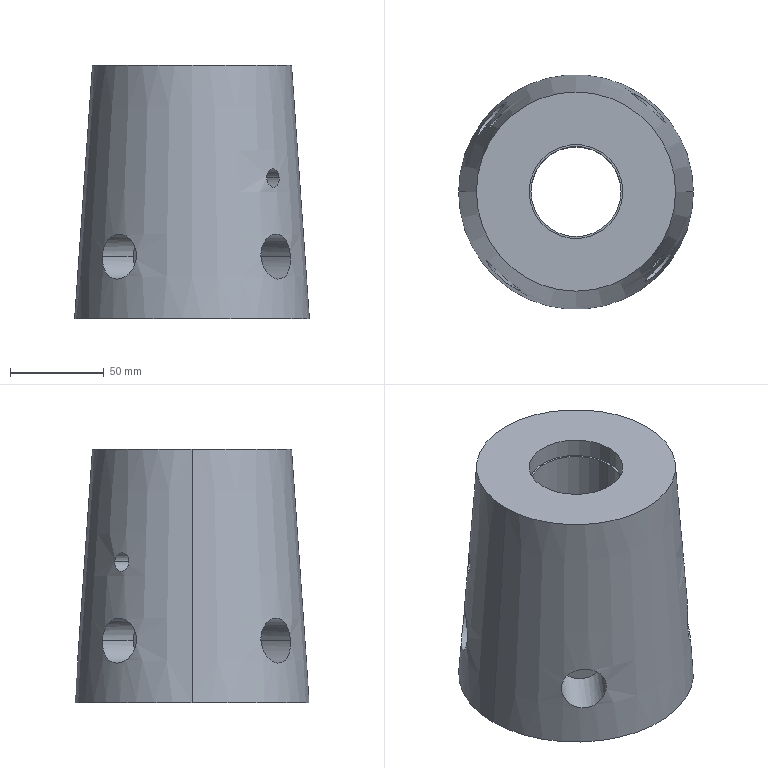Part | SolidWorks | features HoleWzd 7, Revolution 1 | 1 solid | 27 faces | box 125 x 125 x 135 mm | volume 1121518 mm3 | cylinder 16 | plane 9 | cone 2 | commonest cylinder face diameters 24 x8 10 x4 48 x2 50 x2